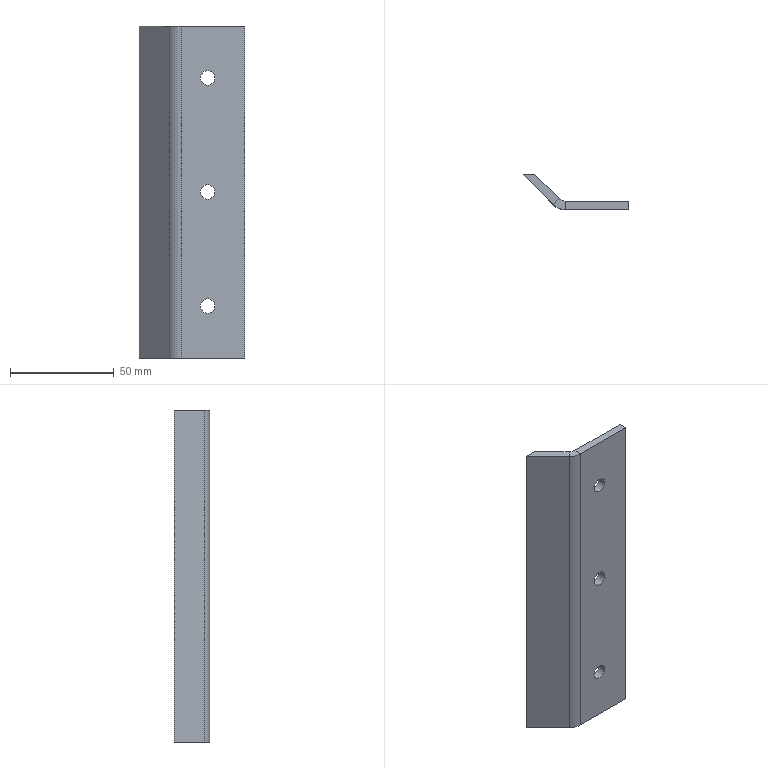Part | SolidWorks | 1 solid | 20 faces | box 51.059 x 17.007 x 160 mm | volume 34219 mm3 | plane 12 | cylinder 8 | commonest cylinder face diameters 7 x6 8 x1 16 x1
STEP:
#1=CARTESIAN_POINT('',(11.5,4.,55.));
#2=VERTEX_POINT('',#1);
#3=CARTESIAN_POINT('',(18.5,4.,55.));
#4=VERTEX_POINT('',#3);
#5=CARTESIAN_POINT('',(15.,4.,55.));
#6=DIRECTION('',(0.,1.,0.));
#7=DIRECTION('',(-1.,0.,0.));
#8=AXIS2_PLACEMENT_3D('',#5,#6,#7);
#9=CIRCLE('',#8,3.5);
#10=EDGE_CURVE('',#2,#4,#9,.T.);
#11=ORIENTED_EDGE('',*,*,#10,.T.);
#12=CARTESIAN_POINT('',(18.5,0.,55.));
#13=VERTEX_POINT('',#12);
#14=CARTESIAN_POINT('',(18.5,4.,55.));
#15=DIRECTION('',(0.,-1.,0.));
#16=VECTOR('',#15,1000.);
#17=LINE('',#14,#16);
#18=EDGE_CURVE('',#4,#13,#17,.T.);
#19=ORIENTED_EDGE('',*,*,#18,.T.);
#20=CARTESIAN_POINT('',(11.5,0.,55.));
#21=VERTEX_POINT('',#20);
#22=CARTESIAN_POINT('',(15.,0.,55.));
#23=DIRECTION('',(0.,-1.,0.));
#24=DIRECTION('',(1.,0.,0.));
#25=AXIS2_PLACEMENT_3D('',#22,#23,#24);
#26=CIRCLE('',#25,3.5);
#27=EDGE_CURVE('',#13,#21,#26,.T.);
#28=ORIENTED_EDGE('',*,*,#27,.T.);
#29=CARTESIAN_POINT('',(11.5,4.,55.));
#30=DIRECTION('',(0.,-1.,0.));
#31=VECTOR('',#30,1000.);
#32=LINE('',#29,#31);
#33=EDGE_CURVE('',#2,#21,#32,.T.);
#34=ORIENTED_EDGE('',*,*,#33,.F.);
#35=EDGE_LOOP('',(#11,#19,#28,#34));
#36=FACE_OUTER_BOUND('',#35,.T.);
#37=CARTESIAN_POINT('',(15.,2.,55.));
#38=DIRECTION('',(0.,1.,0.));
#39=DIRECTION('',(1.,0.,0.));
#40=AXIS2_PLACEMENT_3D('',#37,#38,#39);
#41=CYLINDRICAL_SURFACE('',#40,3.5);
#42=ADVANCED_FACE('',(#36),#41,.F.);
#43=ORIENTED_EDGE('',*,*,#18,.F.);
#44=CARTESIAN_POINT('',(15.,4.,55.));
#45=DIRECTION('',(0.,1.,0.));
#46=DIRECTION('',(1.,0.,0.));
#47=AXIS2_PLACEMENT_3D('',#44,#45,#46);
#48=CIRCLE('',#47,3.5);
#49=EDGE_CURVE('',#4,#2,#48,.T.);
#50=ORIENTED_EDGE('',*,*,#49,.T.);
#51=ORIENTED_EDGE('',*,*,#33,.T.);
#52=CARTESIAN_POINT('',(15.,0.,55.));
#53=DIRECTION('',(0.,-1.,0.));
#54=DIRECTION('',(-1.,0.,0.));
#55=AXIS2_PLACEMENT_3D('',#52,#53,#54);
#56=CIRCLE('',#55,3.5);
#57=EDGE_CURVE('',#21,#13,#56,.T.);
#58=ORIENTED_EDGE('',*,*,#57,.T.);
#59=EDGE_LOOP('',(#43,#50,#51,#58));
#60=FACE_OUTER_BOUND('',#59,.T.);
#61=CARTESIAN_POINT('',(15.,2.,55.));
#62=DIRECTION('',(0.,1.,0.));
#63=DIRECTION('',(1.,0.,0.));
#64=AXIS2_PLACEMENT_3D('',#61,#62,#63);
#65=CYLINDRICAL_SURFACE('',#64,3.5);
#66=ADVANCED_FACE('',(#60),#65,.F.);
#67=CARTESIAN_POINT('',(11.5,4.,-55.));
#68=VERTEX_POINT('',#67);
#69=CARTESIAN_POINT('',(18.5,4.,-55.));
#70=VERTEX_POINT('',#69);
#71=CARTESIAN_POINT('',(15.,4.,-55.));
#72=DIRECTION('',(0.,1.,0.));
#73=DIRECTION('',(-1.,0.,0.));
#74=AXIS2_PLACEMENT_3D('',#71,#72,#73);
#75=CIRCLE('',#74,3.5);
#76=EDGE_CURVE('',#68,#70,#75,.T.);
#77=ORIENTED_EDGE('',*,*,#76,.T.);
#78=CARTESIAN_POINT('',(18.5,0.,-55.));
#79=VERTEX_POINT('',#78);
#80=CARTESIAN_POINT('',(18.5,4.,-55.));
#81=DIRECTION('',(0.,-1.,0.));
#82=VECTOR('',#81,1000.);
#83=LINE('',#80,#82);
#84=EDGE_CURVE('',#70,#79,#83,.T.);
#85=ORIENTED_EDGE('',*,*,#84,.T.);
#86=CARTESIAN_POINT('',(11.5,0.,-55.));
#87=VERTEX_POINT('',#86);
#88=CARTESIAN_POINT('',(15.,0.,-55.));
#89=DIRECTION('',(0.,-1.,0.));
#90=DIRECTION('',(1.,0.,0.));
#91=AXIS2_PLACEMENT_3D('',#88,#89,#90);
#92=CIRCLE('',#91,3.5);
#93=EDGE_CURVE('',#79,#87,#92,.T.);
#94=ORIENTED_EDGE('',*,*,#93,.T.);
#95=CARTESIAN_POINT('',(11.5,4.,-55.));
#96=DIRECTION('',(0.,-1.,0.));
#97=VECTOR('',#96,1000.);
#98=LINE('',#95,#97);
#99=EDGE_CURVE('',#68,#87,#98,.T.);
#100=ORIENTED_EDGE('',*,*,#99,.F.);
#101=EDGE_LOOP('',(#77,#85,#94,#100));
#102=FACE_OUTER_BOUND('',#101,.T.);
#103=CARTESIAN_POINT('',(15.,2.,-55.));
#104=DIRECTION('',(0.,1.,0.));
#105=DIRECTION('',(1.,0.,0.));
#106=AXIS2_PLACEMENT_3D('',#103,#104,#105);
#107=CYLINDRICAL_SURFACE('',#106,3.5);
#108=ADVANCED_FACE('',(#102),#107,.F.);
#109=ORIENTED_EDGE('',*,*,#84,.F.);
#110=CARTESIAN_POINT('',(15.,4.,-55.));
#111=DIRECTION('',(0.,1.,0.));
#112=DIRECTION('',(1.,0.,0.));
#113=AXIS2_PLACEMENT_3D('',#110,#111,#112);
#114=CIRCLE('',#113,3.5);
#115=EDGE_CURVE('',#70,#68,#114,.T.);
#116=ORIENTED_EDGE('',*,*,#115,.T.);
#117=ORIENTED_EDGE('',*,*,#99,.T.);
#118=CARTESIAN_POINT('',(15.,0.,-55.));
#119=DIRECTION('',(0.,-1.,0.));
#120=DIRECTION('',(-1.,0.,0.));
#121=AXIS2_PLACEMENT_3D('',#118,#119,#120);
#122=CIRCLE('',#121,3.5);
#123=EDGE_CURVE('',#87,#79,#122,.T.);
#124=ORIENTED_EDGE('',*,*,#123,.T.);
#125=EDGE_LOOP('',(#109,#116,#117,#124));
#126=FACE_OUTER_BOUND('',#125,.T.);
#127=CARTESIAN_POINT('',(15.,2.,-55.));
#128=DIRECTION('',(0.,1.,0.));
#129=DIRECTION('',(1.,0.,0.));
#130=AXIS2_PLACEMENT_3D('',#127,#128,#129);
#131=CYLINDRICAL_SURFACE('',#130,3.5);
#132=ADVANCED_FACE('',(#126),#131,.F.);
#133=CARTESIAN_POINT('',(11.5,4.,0.));
#134=VERTEX_POINT('',#133);
#135=CARTESIAN_POINT('',(18.5,4.,0.));
#136=VERTEX_POINT('',#135);
#137=CARTESIAN_POINT('',(15.,4.,0.));
#138=DIRECTION('',(0.,1.,0.));
#139=DIRECTION('',(-1.,0.,0.));
#140=AXIS2_PLACEMENT_3D('',#137,#138,#139);
#141=CIRCLE('',#140,3.5);
#142=EDGE_CURVE('',#134,#136,#141,.T.);
#143=ORIENTED_EDGE('',*,*,#142,.T.);
#144=CARTESIAN_POINT('',(18.5,0.,0.));
#145=VERTEX_POINT('',#144);
#146=CARTESIAN_POINT('',(18.5,4.,0.));
#147=DIRECTION('',(0.,-1.,0.));
#148=VECTOR('',#147,1000.);
#149=LINE('',#146,#148);
#150=EDGE_CURVE('',#136,#145,#149,.T.);
#151=ORIENTED_EDGE('',*,*,#150,.T.);
#152=CARTESIAN_POINT('',(11.5,0.,0.));
#153=VERTEX_POINT('',#152);
#154=CARTESIAN_POINT('',(15.,0.,0.));
#155=DIRECTION('',(0.,-1.,0.));
#156=DIRECTION('',(1.,0.,0.));
#157=AXIS2_PLACEMENT_3D('',#154,#155,#156);
#158=CIRCLE('',#157,3.5);
#159=EDGE_CURVE('',#145,#153,#158,.T.);
#160=ORIENTED_EDGE('',*,*,#159,.T.);
#161=CARTESIAN_POINT('',(11.5,4.,0.));
#162=DIRECTION('',(0.,-1.,0.));
#163=VECTOR('',#162,1000.);
#164=LINE('',#161,#163);
#165=EDGE_CURVE('',#134,#153,#164,.T.);
#166=ORIENTED_EDGE('',*,*,#165,.F.);
#167=EDGE_LOOP('',(#143,#151,#160,#166));
#168=FACE_OUTER_BOUND('',#167,.T.);
#169=CARTESIAN_POINT('',(15.,2.,0.));
#170=DIRECTION('',(0.,1.,0.));
#171=DIRECTION('',(1.,0.,0.));
#172=AXIS2_PLACEMENT_3D('',#169,#170,#171);
#173=CYLINDRICAL_SURFACE('',#172,3.5);
#174=ADVANCED_FACE('',(#168),#173,.F.);
#175=ORIENTED_EDGE('',*,*,#150,.F.);
#176=CARTESIAN_POINT('',(15.,4.,0.));
#177=DIRECTION('',(0.,1.,0.));
#178=DIRECTION('',(1.,0.,0.));
#179=AXIS2_PLACEMENT_3D('',#176,#177,#178);
#180=CIRCLE('',#179,3.5);
#181=EDGE_CURVE('',#136,#134,#180,.T.);
#182=ORIENTED_EDGE('',*,*,#181,.T.);
#183=ORIENTED_EDGE('',*,*,#165,.T.);
#184=CARTESIAN_POINT('',(15.,0.,0.));
#185=DIRECTION('',(0.,-1.,0.));
#186=DIRECTION('',(-1.,0.,0.));
#187=AXIS2_PLACEMENT_3D('',#184,#185,#186);
#188=CIRCLE('',#187,3.5);
#189=EDGE_CURVE('',#153,#145,#188,.T.);
#190=ORIENTED_EDGE('',*,*,#189,.T.);
#191=EDGE_LOOP('',(#175,#182,#183,#190));
#192=FACE_OUTER_BOUND('',#191,.T.);
#193=CARTESIAN_POINT('',(15.,2.,0.));
#194=DIRECTION('',(0.,1.,0.));
#195=DIRECTION('',(1.,0.,0.));
#196=AXIS2_PLACEMENT_3D('',#193,#194,#195);
#197=CYLINDRICAL_SURFACE('',#196,3.5);
#198=ADVANCED_FACE('',(#192),#197,.F.);
#199=CARTESIAN_POINT('',(33.,4.,-80.));
#200=VERTEX_POINT('',#199);
#201=CARTESIAN_POINT('',(33.,4.,80.));
#202=VERTEX_POINT('',#201);
#203=CARTESIAN_POINT('',(33.,4.,-80.));
#204=DIRECTION('',(0.,0.,1.));
#205=VECTOR('',#204,1000.);
#206=LINE('',#203,#205);
#207=EDGE_CURVE('',#200,#202,#206,.T.);
#208=ORIENTED_EDGE('',*,*,#207,.T.);
#209=CARTESIAN_POINT('',(33.,0.,80.));
#210=VERTEX_POINT('',#209);
#211=CARTESIAN_POINT('',(33.,0.,80.));
#212=DIRECTION('',(0.,1.,0.));
#213=VECTOR('',#212,1000.);
#214=LINE('',#211,#213);
#215=EDGE_CURVE('',#210,#202,#214,.T.);
#216=ORIENTED_EDGE('',*,*,#215,.F.);
#217=CARTESIAN_POINT('',(33.,0.,-80.));
#218=VERTEX_POINT('',#217);
#219=CARTESIAN_POINT('',(33.,0.,-80.));
#220=DIRECTION('',(0.,0.,1.));
#221=VECTOR('',#220,1000.);
#222=LINE('',#219,#221);
#223=EDGE_CURVE('',#218,#210,#222,.T.);
#224=ORIENTED_EDGE('',*,*,#223,.F.);
#225=CARTESIAN_POINT('',(33.,0.,-80.));
#226=DIRECTION('',(0.,1.,0.));
#227=VECTOR('',#226,1000.);
#228=LINE('',#225,#227);
#229=EDGE_CURVE('',#218,#200,#228,.T.);
#230=ORIENTED_EDGE('',*,*,#229,.T.);
#231=EDGE_LOOP('',(#208,#216,#224,#230));
#232=FACE_OUTER_BOUND('',#231,.T.);
#233=CARTESIAN_POINT('',(33.,4.,80.));
#234=DIRECTION('',(1.,0.,0.));
#235=DIRECTION('',(0.,1.,0.));
#236=AXIS2_PLACEMENT_3D('',#233,#234,#235);
#237=PLANE('',#236);
#238=ADVANCED_FACE('',(#232),#237,.T.);
#239=CARTESIAN_POINT('',(-0.5665,5.172,80.));
#240=VERTEX_POINT('',#239);
#241=CARTESIAN_POINT('',(-3.395,2.343,80.));
#242=VERTEX_POINT('',#241);
#243=CARTESIAN_POINT('',(-0.5665,5.172,80.));
#244=DIRECTION('',(-0.7071,-0.7071,0.));
#245=VECTOR('',#244,1000.);
#246=LINE('',#243,#245);
#247=EDGE_CURVE('',#240,#242,#246,.T.);
#248=ORIENTED_EDGE('',*,*,#247,.F.);
#249=CARTESIAN_POINT('',(-12.402,17.007,80.));
#250=VERTEX_POINT('',#249);
#251=CARTESIAN_POINT('',(-12.402,17.007,80.));
#252=DIRECTION('',(0.7071,-0.7071,0.));
#253=VECTOR('',#252,1000.);
#254=LINE('',#251,#253);
#255=EDGE_CURVE('',#250,#240,#254,.T.);
#256=ORIENTED_EDGE('',*,*,#255,.F.);
#257=CARTESIAN_POINT('',(-18.059,17.007,80.));
#258=VERTEX_POINT('',#257);
#259=CARTESIAN_POINT('',(-12.402,17.007,80.));
#260=DIRECTION('',(-1.,0.,0.));
#261=VECTOR('',#260,1000.);
#262=LINE('',#259,#261);
#263=EDGE_CURVE('',#250,#258,#262,.T.);
#264=ORIENTED_EDGE('',*,*,#263,.T.);
#265=CARTESIAN_POINT('',(-3.395,2.343,80.));
#266=DIRECTION('',(-0.7071,0.7071,0.));
#267=VECTOR('',#266,1000.);
#268=LINE('',#265,#267);
#269=EDGE_CURVE('',#242,#258,#268,.T.);
#270=ORIENTED_EDGE('',*,*,#269,.F.);
#271=EDGE_LOOP('',(#248,#256,#264,#270));
#272=FACE_OUTER_BOUND('',#271,.T.);
#273=CARTESIAN_POINT('',(14.468,-15.52,80.));
#274=DIRECTION('',(0.,0.,1.));
#275=DIRECTION('',(1.,0.,0.));
#276=AXIS2_PLACEMENT_3D('',#273,#274,#275);
#277=PLANE('',#276);
#278=ADVANCED_FACE('',(#272),#277,.T.);
#279=CARTESIAN_POINT('',(2.262,4.,-80.));
#280=VERTEX_POINT('',#279);
#281=CARTESIAN_POINT('',(-0.5665,5.172,-80.));
#282=VERTEX_POINT('',#281);
#283=CARTESIAN_POINT('',(2.262,8.,-80.));
#284=DIRECTION('',(0.,0.,-1.));
#285=DIRECTION('',(0.,-1.,0.));
#286=AXIS2_PLACEMENT_3D('',#283,#284,#285);
#287=CIRCLE('',#286,4.);
#288=EDGE_CURVE('',#280,#282,#287,.T.);
#289=ORIENTED_EDGE('',*,*,#288,.T.);
#290=CARTESIAN_POINT('',(-0.5665,5.172,80.));
#291=DIRECTION('',(0.,0.,-1.));
#292=VECTOR('',#291,1000.);
#293=LINE('',#290,#292);
#294=EDGE_CURVE('',#240,#282,#293,.T.);
#295=ORIENTED_EDGE('',*,*,#294,.F.);
#296=CARTESIAN_POINT('',(2.262,4.,80.));
#297=VERTEX_POINT('',#296);
#298=CARTESIAN_POINT('',(2.262,8.,80.));
#299=DIRECTION('',(0.,0.,1.));
#300=DIRECTION('',(-0.7071,-0.7071,0.));
#301=AXIS2_PLACEMENT_3D('',#298,#299,#300);
#302=CIRCLE('',#301,4.);
#303=EDGE_CURVE('',#240,#297,#302,.T.);
#304=ORIENTED_EDGE('',*,*,#303,.T.);
#305=CARTESIAN_POINT('',(2.262,4.,-80.));
#306=DIRECTION('',(0.,0.,1.));
#307=VECTOR('',#306,1000.);
#308=LINE('',#305,#307);
#309=EDGE_CURVE('',#280,#297,#308,.T.);
#310=ORIENTED_EDGE('',*,*,#309,.F.);
#311=EDGE_LOOP('',(#289,#295,#304,#310));
#312=FACE_OUTER_BOUND('',#311,.T.);
#313=CARTESIAN_POINT('',(2.262,8.,0.));
#314=DIRECTION('',(0.,0.,-1.));
#315=DIRECTION('',(0.,-1.,0.));
#316=AXIS2_PLACEMENT_3D('',#313,#314,#315);
#317=CYLINDRICAL_SURFACE('',#316,4.);
#318=ADVANCED_FACE('',(#312),#317,.F.);
#319=ORIENTED_EDGE('',*,*,#288,.F.);
#320=CARTESIAN_POINT('',(2.262,0.,-80.));
#321=VERTEX_POINT('',#320);
#322=CARTESIAN_POINT('',(2.262,4.,-80.));
#323=DIRECTION('',(0.,-1.,0.));
#324=VECTOR('',#323,1000.);
#325=LINE('',#322,#324);
#326=EDGE_CURVE('',#280,#321,#325,.T.);
#327=ORIENTED_EDGE('',*,*,#326,.T.);
#328=CARTESIAN_POINT('',(-3.395,2.343,-80.));
#329=VERTEX_POINT('',#328);
#330=CARTESIAN_POINT('',(2.262,8.,-80.));
#331=DIRECTION('',(0.,0.,1.));
#332=DIRECTION('',(-0.7071,-0.7071,0.));
#333=AXIS2_PLACEMENT_3D('',#330,#331,#332);
#334=CIRCLE('',#333,8.);
#335=EDGE_CURVE('',#329,#321,#334,.T.);
#336=ORIENTED_EDGE('',*,*,#335,.F.);
#337=CARTESIAN_POINT('',(-3.395,2.343,-80.));
#338=DIRECTION('',(0.7071,0.7071,0.));
#339=VECTOR('',#338,1000.);
#340=LINE('',#337,#339);
#341=EDGE_CURVE('',#329,#282,#340,.T.);
#342=ORIENTED_EDGE('',*,*,#341,.T.);
#343=EDGE_LOOP('',(#319,#327,#336,#342));
#344=FACE_OUTER_BOUND('',#343,.T.);
#345=CARTESIAN_POINT('',(2.262,-7.,-80.));
#346=DIRECTION('',(0.,0.,-1.));
#347=DIRECTION('',(-1.,0.,0.));
#348=AXIS2_PLACEMENT_3D('',#345,#346,#347);
#349=PLANE('',#348);
#350=ADVANCED_FACE('',(#344),#349,.T.);
#351=ORIENTED_EDGE('',*,*,#341,.F.);
#352=CARTESIAN_POINT('',(-18.059,17.007,-80.));
#353=VERTEX_POINT('',#352);
#354=CARTESIAN_POINT('',(-18.059,17.007,-80.));
#355=DIRECTION('',(0.7071,-0.7071,0.));
#356=VECTOR('',#355,1000.);
#357=LINE('',#354,#356);
#358=EDGE_CURVE('',#353,#329,#357,.T.);
#359=ORIENTED_EDGE('',*,*,#358,.F.);
#360=CARTESIAN_POINT('',(-12.402,17.007,-80.));
#361=VERTEX_POINT('',#360);
#362=CARTESIAN_POINT('',(-18.059,17.007,-80.));
#363=DIRECTION('',(1.,0.,0.));
#364=VECTOR('',#363,1000.);
#365=LINE('',#362,#364);
#366=EDGE_CURVE('',#353,#361,#365,.T.);
#367=ORIENTED_EDGE('',*,*,#366,.T.);
#368=CARTESIAN_POINT('',(-0.5665,5.172,-80.));
#369=DIRECTION('',(-0.7071,0.7071,0.));
#370=VECTOR('',#369,1000.);
#371=LINE('',#368,#370);
#372=EDGE_CURVE('',#282,#361,#371,.T.);
#373=ORIENTED_EDGE('',*,*,#372,.F.);
#374=EDGE_LOOP('',(#351,#359,#367,#373));
#375=FACE_OUTER_BOUND('',#374,.T.);
#376=CARTESIAN_POINT('',(-18.059,17.007,-80.));
#377=DIRECTION('',(0.,0.,-1.));
#378=DIRECTION('',(0.,-1.,0.));
#379=AXIS2_PLACEMENT_3D('',#376,#377,#378);
#380=PLANE('',#379);
#381=ADVANCED_FACE('',(#375),#380,.T.);
#382=ORIENTED_EDGE('',*,*,#255,.T.);
#383=ORIENTED_EDGE('',*,*,#294,.T.);
#384=ORIENTED_EDGE('',*,*,#372,.T.);
#385=CARTESIAN_POINT('',(-12.402,17.007,-80.));
#386=DIRECTION('',(0.,0.,1.));
#387=VECTOR('',#386,1000.);
#388=LINE('',#385,#387);
#389=EDGE_CURVE('',#361,#250,#388,.T.);
#390=ORIENTED_EDGE('',*,*,#389,.T.);
#391=EDGE_LOOP('',(#382,#383,#384,#390));
#392=FACE_OUTER_BOUND('',#391,.T.);
#393=CARTESIAN_POINT('',(1.033,3.572,0.));
#394=DIRECTION('',(0.7071,0.7071,0.));
#395=DIRECTION('',(0.,0.,-1.));
#396=AXIS2_PLACEMENT_3D('',#393,#394,#395);
#397=PLANE('',#396);
#398=ADVANCED_FACE('',(#392),#397,.T.);
#399=ORIENTED_EDGE('',*,*,#366,.F.);
#400=CARTESIAN_POINT('',(-18.059,17.007,80.));
#401=DIRECTION('',(0.,0.,-1.));
#402=VECTOR('',#401,1000.);
#403=LINE('',#400,#402);
#404=EDGE_CURVE('',#258,#353,#403,.T.);
#405=ORIENTED_EDGE('',*,*,#404,.F.);
#406=ORIENTED_EDGE('',*,*,#263,.F.);
#407=ORIENTED_EDGE('',*,*,#389,.F.);
#408=EDGE_LOOP('',(#399,#405,#406,#407));
#409=FACE_OUTER_BOUND('',#408,.T.);
#410=CARTESIAN_POINT('',(-15.23,17.007,40.));
#411=DIRECTION('',(0.,1.,0.));
#412=DIRECTION('',(1.,0.,0.));
#413=AXIS2_PLACEMENT_3D('',#410,#411,#412);
#414=PLANE('',#413);
#415=ADVANCED_FACE('',(#409),#414,.T.);
#416=ORIENTED_EDGE('',*,*,#358,.T.);
#417=CARTESIAN_POINT('',(-3.395,2.343,-80.));
#418=DIRECTION('',(0.,0.,1.));
#419=VECTOR('',#418,1000.);
#420=LINE('',#417,#419);
#421=EDGE_CURVE('',#329,#242,#420,.T.);
#422=ORIENTED_EDGE('',*,*,#421,.T.);
#423=ORIENTED_EDGE('',*,*,#269,.T.);
#424=ORIENTED_EDGE('',*,*,#404,.T.);
#425=EDGE_LOOP('',(#416,#422,#423,#424));
#426=FACE_OUTER_BOUND('',#425,.T.);
#427=CARTESIAN_POINT('',(-1.795,0.7437,0.));
#428=DIRECTION('',(0.7071,0.7071,0.));
#429=DIRECTION('',(0.,0.,-1.));
#430=AXIS2_PLACEMENT_3D('',#427,#428,#429);
#431=PLANE('',#430);
#432=ADVANCED_FACE('',(#426),#431,.F.);
#433=ORIENTED_EDGE('',*,*,#335,.T.);
#434=CARTESIAN_POINT('',(2.262,0.,80.));
#435=VERTEX_POINT('',#434);
#436=CARTESIAN_POINT('',(2.262,0.,80.));
#437=DIRECTION('',(0.,0.,-1.));
#438=VECTOR('',#437,1000.);
#439=LINE('',#436,#438);
#440=EDGE_CURVE('',#435,#321,#439,.T.);
#441=ORIENTED_EDGE('',*,*,#440,.F.);
#442=CARTESIAN_POINT('',(2.262,8.,80.));
#443=DIRECTION('',(0.,0.,-1.));
#444=DIRECTION('',(0.,-1.,0.));
#445=AXIS2_PLACEMENT_3D('',#442,#443,#444);
#446=CIRCLE('',#445,8.);
#447=EDGE_CURVE('',#435,#242,#446,.T.);
#448=ORIENTED_EDGE('',*,*,#447,.T.);
#449=ORIENTED_EDGE('',*,*,#421,.F.);
#450=EDGE_LOOP('',(#433,#441,#448,#449));
#451=FACE_OUTER_BOUND('',#450,.T.);
#452=CARTESIAN_POINT('',(2.262,8.,0.));
#453=DIRECTION('',(0.,0.,-1.));
#454=DIRECTION('',(0.,-1.,0.));
#455=AXIS2_PLACEMENT_3D('',#452,#453,#454);
#456=CYLINDRICAL_SURFACE('',#455,8.);
#457=ADVANCED_FACE('',(#451),#456,.T.);
#458=ORIENTED_EDGE('',*,*,#303,.F.);
#459=ORIENTED_EDGE('',*,*,#247,.T.);
#460=ORIENTED_EDGE('',*,*,#447,.F.);
#461=CARTESIAN_POINT('',(2.262,0.,80.));
#462=DIRECTION('',(0.,1.,0.));
#463=VECTOR('',#462,1000.);
#464=LINE('',#461,#463);
#465=EDGE_CURVE('',#435,#297,#464,.T.);
#466=ORIENTED_EDGE('',*,*,#465,.T.);
#467=EDGE_LOOP('',(#458,#459,#460,#466));
#468=FACE_OUTER_BOUND('',#467,.T.);
#469=CARTESIAN_POINT('',(2.262,-7.,80.));
#470=DIRECTION('',(0.,0.,-1.));
#471=DIRECTION('',(0.,-1.,0.));
#472=AXIS2_PLACEMENT_3D('',#469,#470,#471);
#473=PLANE('',#472);
#474=ADVANCED_FACE('',(#468),#473,.F.);
#475=ORIENTED_EDGE('',*,*,#215,.T.);
#476=CARTESIAN_POINT('',(2.262,4.,80.));
#477=DIRECTION('',(1.,0.,0.));
#478=VECTOR('',#477,1000.);
#479=LINE('',#476,#478);
#480=EDGE_CURVE('',#297,#202,#479,.T.);
#481=ORIENTED_EDGE('',*,*,#480,.F.);
#482=ORIENTED_EDGE('',*,*,#465,.F.);
#483=CARTESIAN_POINT('',(2.262,0.,80.));
#484=DIRECTION('',(1.,0.,0.));
#485=VECTOR('',#484,1000.);
#486=LINE('',#483,#485);
#487=EDGE_CURVE('',#435,#210,#486,.T.);
#488=ORIENTED_EDGE('',*,*,#487,.T.);
#489=EDGE_LOOP('',(#475,#481,#482,#488));
#490=FACE_OUTER_BOUND('',#489,.T.);
#491=CARTESIAN_POINT('',(23.,0.,80.));
#492=DIRECTION('',(0.,0.,1.));
#493=DIRECTION('',(1.,0.,0.));
#494=AXIS2_PLACEMENT_3D('',#491,#492,#493);
#495=PLANE('',#494);
#496=ADVANCED_FACE('',(#490),#495,.T.);
#497=ORIENTED_EDGE('',*,*,#10,.F.);
#498=ORIENTED_EDGE('',*,*,#49,.F.);
#499=EDGE_LOOP('',(#497,#498));
#500=FACE_BOUND('',#499,.T.);
#501=ORIENTED_EDGE('',*,*,#76,.F.);
#502=ORIENTED_EDGE('',*,*,#115,.F.);
#503=EDGE_LOOP('',(#501,#502));
#504=FACE_BOUND('',#503,.T.);
#505=ORIENTED_EDGE('',*,*,#142,.F.);
#506=ORIENTED_EDGE('',*,*,#181,.F.);
#507=EDGE_LOOP('',(#505,#506));
#508=FACE_BOUND('',#507,.T.);
#509=ORIENTED_EDGE('',*,*,#207,.F.);
#510=CARTESIAN_POINT('',(2.262,4.,-80.));
#511=DIRECTION('',(1.,0.,0.));
#512=VECTOR('',#511,1000.);
#513=LINE('',#510,#512);
#514=EDGE_CURVE('',#280,#200,#513,.T.);
#515=ORIENTED_EDGE('',*,*,#514,.F.);
#516=ORIENTED_EDGE('',*,*,#309,.T.);
#517=ORIENTED_EDGE('',*,*,#480,.T.);
#518=EDGE_LOOP('',(#509,#515,#516,#517));
#519=FACE_OUTER_BOUND('',#518,.T.);
#520=CARTESIAN_POINT('',(0.,4.,0.));
#521=DIRECTION('',(0.,1.,0.));
#522=DIRECTION('',(1.,0.,0.));
#523=AXIS2_PLACEMENT_3D('',#520,#521,#522);
#524=PLANE('',#523);
#525=ADVANCED_FACE('',(#500,#504,#508,#519),#524,.T.);
#526=ORIENTED_EDGE('',*,*,#229,.F.);
#527=CARTESIAN_POINT('',(33.,0.,-80.));
#528=DIRECTION('',(-1.,0.,0.));
#529=VECTOR('',#528,1000.);
#530=LINE('',#527,#529);
#531=EDGE_CURVE('',#218,#321,#530,.T.);
#532=ORIENTED_EDGE('',*,*,#531,.T.);
#533=ORIENTED_EDGE('',*,*,#326,.F.);
#534=ORIENTED_EDGE('',*,*,#514,.T.);
#535=EDGE_LOOP('',(#526,#532,#533,#534));
#536=FACE_OUTER_BOUND('',#535,.T.);
#537=CARTESIAN_POINT('',(-23.,0.,-80.));
#538=DIRECTION('',(0.,0.,-1.));
#539=DIRECTION('',(0.,-1.,0.));
#540=AXIS2_PLACEMENT_3D('',#537,#538,#539);
#541=PLANE('',#540);
#542=ADVANCED_FACE('',(#536),#541,.T.);
#543=ORIENTED_EDGE('',*,*,#189,.F.);
#544=ORIENTED_EDGE('',*,*,#159,.F.);
#545=EDGE_LOOP('',(#543,#544));
#546=FACE_BOUND('',#545,.T.);
#547=ORIENTED_EDGE('',*,*,#123,.F.);
#548=ORIENTED_EDGE('',*,*,#93,.F.);
#549=EDGE_LOOP('',(#547,#548));
#550=FACE_BOUND('',#549,.T.);
#551=ORIENTED_EDGE('',*,*,#57,.F.);
#552=ORIENTED_EDGE('',*,*,#27,.F.);
#553=EDGE_LOOP('',(#551,#552));
#554=FACE_BOUND('',#553,.T.);
#555=ORIENTED_EDGE('',*,*,#223,.T.);
#556=ORIENTED_EDGE('',*,*,#487,.F.);
#557=ORIENTED_EDGE('',*,*,#440,.T.);
#558=ORIENTED_EDGE('',*,*,#531,.F.);
#559=EDGE_LOOP('',(#555,#556,#557,#558));
#560=FACE_OUTER_BOUND('',#559,.T.);
#561=CARTESIAN_POINT('',(0.,0.,0.));
#562=DIRECTION('',(0.,1.,0.));
#563=DIRECTION('',(1.,0.,0.));
#564=AXIS2_PLACEMENT_3D('',#561,#562,#563);
#565=PLANE('',#564);
#566=ADVANCED_FACE('',(#546,#550,#554,#560),#565,.F.);
#567=CLOSED_SHELL('',(#42,#66,#108,#132,#174,#198,#238,#278,#318,#350,#381,#398,#415,#432,#457,#474,#496,#525,#542,#566));
#568=MANIFOLD_SOLID_BREP('',#567);
#569=CARTESIAN_POINT('',(0.,0.,0.));
#570=DIRECTION('',(0.,0.,1.));
#571=DIRECTION('',(1.,0.,0.));
#572=AXIS2_PLACEMENT_3D('',#569,#570,#571);
#573=(LENGTH_UNIT()NAMED_UNIT(*)SI_UNIT(.MILLI.,.METRE.));
#574=UNCERTAINTY_MEASURE_WITH_UNIT(LENGTH_MEASURE(0.00001),#573,'','');
#575=(NAMED_UNIT(*)PLANE_ANGLE_UNIT()SI_UNIT($,.RADIAN.));
#576=(NAMED_UNIT(*)SI_UNIT($,.STERADIAN.)SOLID_ANGLE_UNIT());
#577=(GEOMETRIC_REPRESENTATION_CONTEXT(3)GLOBAL_UNCERTAINTY_ASSIGNED_CONTEXT((#574))GLOBAL_UNIT_ASSIGNED_CONTEXT((#573,#575,#576))REPRESENTATION_CONTEXT('',''));
#578=ADVANCED_BREP_SHAPE_REPRESENTATION('',(#568,#572),#577);